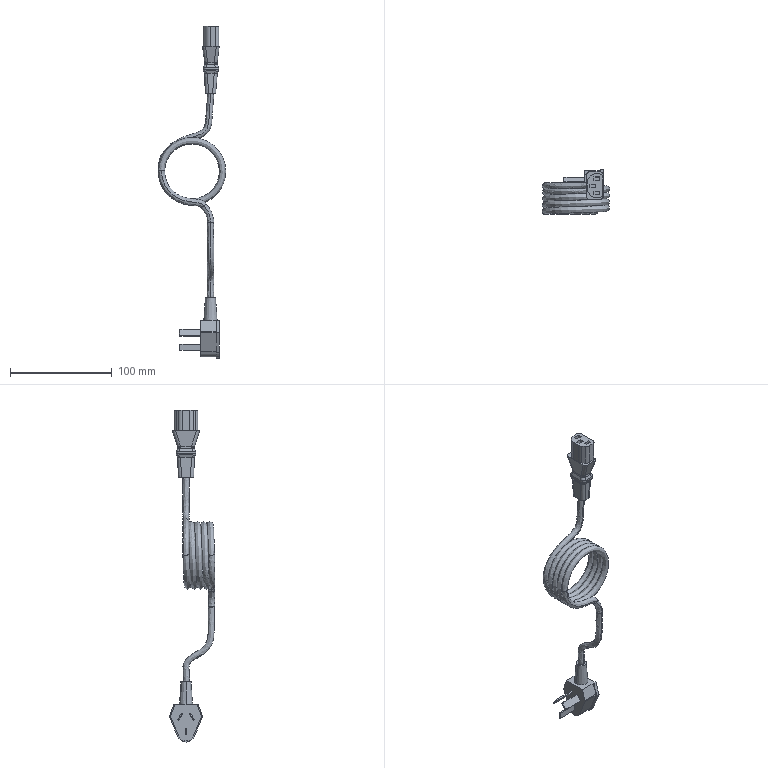Part | SolidWorks | features MirrorStock 1 | 1 solid | 148 faces | box 66.481 x 44.258 x 325.5 mm | volume 63656 mm3 | plane 75 | cylinder 44 | spline 27 | cone 2 | commonest cylinder face diameters 6 x30 1 x6 10 x4 16 x2 18 x2